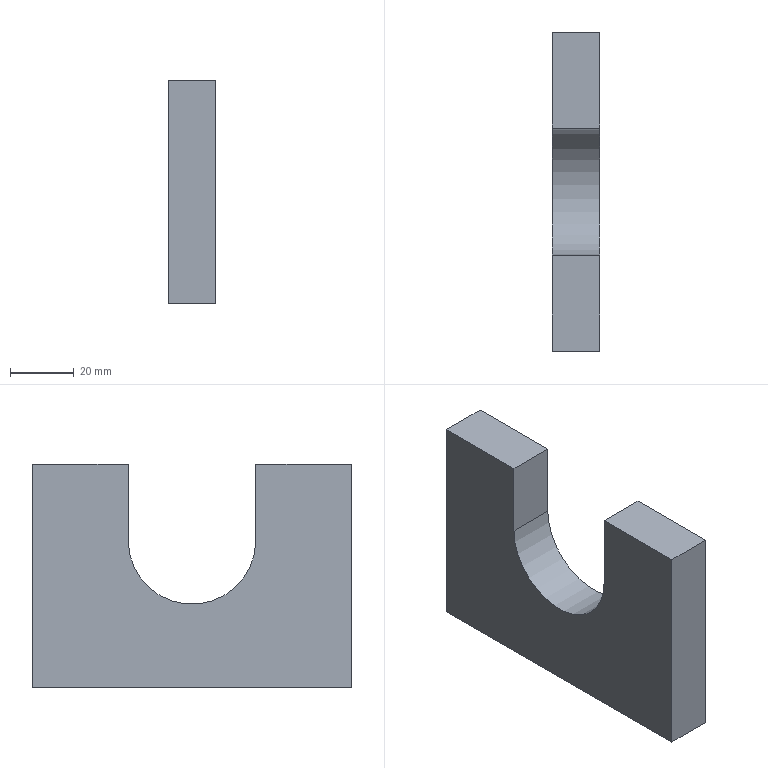Part | STEP file | Tube feed_id678_x_t | 1 solid | 10 faces | box 15 x 100 x 70 mm | volume 81265 mm3 | plane 9 | cylinder 1 | commonest cylinder face diameters 40 x1
STEP:
#1=CARTESIAN_POINT('',(0.,0.,0.));
#2=DIRECTION('',(0.,0.,1.));
#3=DIRECTION('',(1.,0.,0.));
#4=AXIS2_PLACEMENT_3D('',#1,#2,#3);
#5=CARTESIAN_POINT('',(211.,190.936,-4.));
#6=VERTEX_POINT('',#5);
#7=CARTESIAN_POINT('',(211.,190.936,19.85));
#8=VERTEX_POINT('',#7);
#9=CARTESIAN_POINT('',(211.,190.936,12.));
#10=DIRECTION('',(0.,0.,1.));
#11=VECTOR('',#10,1.);
#12=LINE('',#9,#11);
#13=CARTESIAN_POINT('',(211.,245.936,19.85));
#14=DIRECTION('',(1.,0.,0.));
#15=DIRECTION('',(0.,0.,-1.));
#16=AXIS2_PLACEMENT_3D('',#13,#14,#15);
#17=PLANE('',#16);
#18=CARTESIAN_POINT('',(7.85,-55.));
#19=DIRECTION('',(-1.,0.));
#20=VECTOR('',#19,1.);
#21=LINE('',#18,#20);
#22=(GEOMETRIC_REPRESENTATION_CONTEXT(2)PARAMETRIC_REPRESENTATION_CONTEXT()REPRESENTATION_CONTEXT('',''));
#23=DEFINITIONAL_REPRESENTATION('',(#21),#22);
#24=PCURVE('',#17,#23);
#25=CARTESIAN_POINT('',(218.5,190.936,12.));
#26=DIRECTION('',(0.,-1.,0.));
#27=DIRECTION('',(0.,0.,-1.));
#28=AXIS2_PLACEMENT_3D('',#25,#26,#27);
#29=PLANE('',#28);
#30=CARTESIAN_POINT('',(0.,-7.5));
#31=DIRECTION('',(-1.,0.));
#32=VECTOR('',#31,1.);
#33=LINE('',#30,#32);
#34=(GEOMETRIC_REPRESENTATION_CONTEXT(2)PARAMETRIC_REPRESENTATION_CONTEXT()REPRESENTATION_CONTEXT('',''));
#35=DEFINITIONAL_REPRESENTATION('',(#33),#34);
#36=PCURVE('',#29,#35);
#37=SURFACE_CURVE('',#12,(#24,#36),.PCURVE_S1.);
#38=EDGE_CURVE('',#6,#8,#37,.T.);
#39=ORIENTED_EDGE('',*,*,#38,.F.);
#40=CARTESIAN_POINT('',(211.,230.936,-4.));
#41=VERTEX_POINT('',#40);
#42=CARTESIAN_POINT('',(211.,210.936,-4.));
#43=DIRECTION('',(-1.,0.,0.));
#44=DIRECTION('',(0.,0.,-1.));
#45=AXIS2_PLACEMENT_3D('',#42,#43,#44);
#46=CIRCLE('',#45,20.);
#47=CARTESIAN_POINT('',(43.85,-35.));
#48=CARTESIAN_POINT('',(43.85,-69.641));
#49=CARTESIAN_POINT('',(13.85,-52.321));
#50=CARTESIAN_POINT('',(-16.15,-35.));
#51=CARTESIAN_POINT('',(13.85,-17.679));
#52=CARTESIAN_POINT('',(43.85,-0.359));
#53=CARTESIAN_POINT('',(43.85,-35.));
#54=(BOUNDED_CURVE()B_SPLINE_CURVE(2,(#47,#48,#49,#50,#51,#52,#53),.UNSPECIFIED.,.T.,.F.)B_SPLINE_CURVE_WITH_KNOTS((1,2,2,2,2,1),(-2.094,0.,2.094,4.189,6.283,8.378),.UNSPECIFIED.)CURVE()GEOMETRIC_REPRESENTATION_ITEM()RATIONAL_B_SPLINE_CURVE((1.,0.5,1.,0.5,1.,0.5,1.))REPRESENTATION_ITEM(''));
#55=(GEOMETRIC_REPRESENTATION_CONTEXT(2)PARAMETRIC_REPRESENTATION_CONTEXT()REPRESENTATION_CONTEXT('',''));
#56=DEFINITIONAL_REPRESENTATION('',(#54),#55);
#57=PCURVE('',#17,#56);
#58=CARTESIAN_POINT('',(211.,210.936,-4.));
#59=DIRECTION('',(1.,0.,0.));
#60=DIRECTION('',(0.,0.,-1.));
#61=AXIS2_PLACEMENT_3D('',#58,#59,#60);
#62=CYLINDRICAL_SURFACE('',#61,20.);
#63=CARTESIAN_POINT('',(12.566,0.));
#64=DIRECTION('',(-1.,0.));
#65=VECTOR('',#64,1.);
#66=LINE('',#63,#65);
#67=(GEOMETRIC_REPRESENTATION_CONTEXT(2)PARAMETRIC_REPRESENTATION_CONTEXT()REPRESENTATION_CONTEXT('',''));
#68=DEFINITIONAL_REPRESENTATION('',(#66),#67);
#69=PCURVE('',#62,#68);
#70=SURFACE_CURVE('',#46,(#57,#69),.PCURVE_S1.);
#71=EDGE_CURVE('',#41,#6,#70,.T.);
#72=ORIENTED_EDGE('',*,*,#71,.F.);
#73=CARTESIAN_POINT('',(211.,230.936,19.85));
#74=VERTEX_POINT('',#73);
#75=CARTESIAN_POINT('',(211.,230.936,19.85));
#76=DIRECTION('',(0.,0.,1.));
#77=VECTOR('',#76,1.);
#78=LINE('',#75,#77);
#79=CARTESIAN_POINT('',(0.,-15.));
#80=DIRECTION('',(-1.,0.));
#81=VECTOR('',#80,1.);
#82=LINE('',#79,#81);
#83=(GEOMETRIC_REPRESENTATION_CONTEXT(2)PARAMETRIC_REPRESENTATION_CONTEXT()REPRESENTATION_CONTEXT('',''));
#84=DEFINITIONAL_REPRESENTATION('',(#82),#83);
#85=PCURVE('',#17,#84);
#86=CARTESIAN_POINT('',(218.5,230.936,12.));
#87=DIRECTION('',(0.,1.,0.));
#88=DIRECTION('',(0.,0.,1.));
#89=AXIS2_PLACEMENT_3D('',#86,#87,#88);
#90=PLANE('',#89);
#91=CARTESIAN_POINT('',(7.85,-7.5));
#92=DIRECTION('',(1.,0.));
#93=VECTOR('',#92,1.);
#94=LINE('',#91,#93);
#95=(GEOMETRIC_REPRESENTATION_CONTEXT(2)PARAMETRIC_REPRESENTATION_CONTEXT()REPRESENTATION_CONTEXT('',''));
#96=DEFINITIONAL_REPRESENTATION('',(#94),#95);
#97=PCURVE('',#90,#96);
#98=SURFACE_CURVE('',#78,(#85,#97),.PCURVE_S1.);
#99=EDGE_CURVE('',#41,#74,#98,.T.);
#100=ORIENTED_EDGE('',*,*,#99,.T.);
#101=CARTESIAN_POINT('',(211.,260.936,19.85));
#102=VERTEX_POINT('',#101);
#103=CARTESIAN_POINT('',(211.,175.936,19.85));
#104=DIRECTION('',(0.,-1.,0.));
#105=VECTOR('',#104,1.);
#106=LINE('',#103,#105);
#107=CARTESIAN_POINT('',(0.,-70.));
#108=DIRECTION('',(0.,-1.));
#109=VECTOR('',#108,1.);
#110=LINE('',#107,#109);
#111=(GEOMETRIC_REPRESENTATION_CONTEXT(2)PARAMETRIC_REPRESENTATION_CONTEXT()REPRESENTATION_CONTEXT('',''));
#112=DEFINITIONAL_REPRESENTATION('',(#110),#111);
#113=PCURVE('',#17,#112);
#114=CARTESIAN_POINT('',(0.,0.,19.85));
#115=DIRECTION('',(0.,0.,1.));
#116=DIRECTION('',(1.,0.,0.));
#117=AXIS2_PLACEMENT_3D('',#114,#115,#116);
#118=PLANE('',#117);
#119=CARTESIAN_POINT('',(211.,175.936));
#120=DIRECTION('',(0.,-1.));
#121=VECTOR('',#120,1.);
#122=LINE('',#119,#121);
#123=(GEOMETRIC_REPRESENTATION_CONTEXT(2)PARAMETRIC_REPRESENTATION_CONTEXT()REPRESENTATION_CONTEXT('',''));
#124=DEFINITIONAL_REPRESENTATION('',(#122),#123);
#125=PCURVE('',#118,#124);
#126=SURFACE_CURVE('',#106,(#113,#125),.PCURVE_S1.);
#127=EDGE_CURVE('',#102,#74,#126,.T.);
#128=ORIENTED_EDGE('',*,*,#127,.F.);
#129=CARTESIAN_POINT('',(211.,260.936,-50.15));
#130=VERTEX_POINT('',#129);
#131=CARTESIAN_POINT('',(211.,260.936,19.85));
#132=DIRECTION('',(0.,0.,-1.));
#133=VECTOR('',#132,1.);
#134=LINE('',#131,#133);
#135=CARTESIAN_POINT('',(0.,15.));
#136=DIRECTION('',(1.,0.));
#137=VECTOR('',#136,1.);
#138=LINE('',#135,#137);
#139=(GEOMETRIC_REPRESENTATION_CONTEXT(2)PARAMETRIC_REPRESENTATION_CONTEXT()REPRESENTATION_CONTEXT('',''));
#140=DEFINITIONAL_REPRESENTATION('',(#138),#139);
#141=PCURVE('',#17,#140);
#142=CARTESIAN_POINT('',(226.,260.936,19.85));
#143=DIRECTION('',(0.,-1.,0.));
#144=DIRECTION('',(0.,0.,-1.));
#145=AXIS2_PLACEMENT_3D('',#142,#143,#144);
#146=PLANE('',#145);
#147=CARTESIAN_POINT('',(0.,-15.));
#148=DIRECTION('',(1.,0.));
#149=VECTOR('',#148,1.);
#150=LINE('',#147,#149);
#151=(GEOMETRIC_REPRESENTATION_CONTEXT(2)PARAMETRIC_REPRESENTATION_CONTEXT()REPRESENTATION_CONTEXT('',''));
#152=DEFINITIONAL_REPRESENTATION('',(#150),#151);
#153=PCURVE('',#146,#152);
#154=SURFACE_CURVE('',#134,(#141,#153),.PCURVE_S1.);
#155=EDGE_CURVE('',#102,#130,#154,.T.);
#156=ORIENTED_EDGE('',*,*,#155,.T.);
#157=CARTESIAN_POINT('',(211.,160.936,-50.15));
#158=VERTEX_POINT('',#157);
#159=CARTESIAN_POINT('',(211.,245.936,-50.15));
#160=DIRECTION('',(0.,-1.,0.));
#161=VECTOR('',#160,1.);
#162=LINE('',#159,#161);
#163=CARTESIAN_POINT('',(70.,0.));
#164=DIRECTION('',(0.,-1.));
#165=VECTOR('',#164,1.);
#166=LINE('',#163,#165);
#167=(GEOMETRIC_REPRESENTATION_CONTEXT(2)PARAMETRIC_REPRESENTATION_CONTEXT()REPRESENTATION_CONTEXT('',''));
#168=DEFINITIONAL_REPRESENTATION('',(#166),#167);
#169=PCURVE('',#17,#168);
#170=CARTESIAN_POINT('',(0.,0.,-50.15));
#171=DIRECTION('',(0.,0.,1.));
#172=DIRECTION('',(1.,0.,0.));
#173=AXIS2_PLACEMENT_3D('',#170,#171,#172);
#174=PLANE('',#173);
#175=CARTESIAN_POINT('',(211.,245.936));
#176=DIRECTION('',(0.,-1.));
#177=VECTOR('',#176,1.);
#178=LINE('',#175,#177);
#179=(GEOMETRIC_REPRESENTATION_CONTEXT(2)PARAMETRIC_REPRESENTATION_CONTEXT()REPRESENTATION_CONTEXT('',''));
#180=DEFINITIONAL_REPRESENTATION('',(#178),#179);
#181=PCURVE('',#174,#180);
#182=SURFACE_CURVE('',#162,(#169,#181),.PCURVE_S1.);
#183=EDGE_CURVE('',#130,#158,#182,.T.);
#184=ORIENTED_EDGE('',*,*,#183,.T.);
#185=CARTESIAN_POINT('',(211.,160.936,19.85));
#186=VERTEX_POINT('',#185);
#187=CARTESIAN_POINT('',(211.,160.936,19.85));
#188=DIRECTION('',(0.,0.,-1.));
#189=VECTOR('',#188,1.);
#190=LINE('',#187,#189);
#191=CARTESIAN_POINT('',(0.,-85.));
#192=DIRECTION('',(1.,0.));
#193=VECTOR('',#192,1.);
#194=LINE('',#191,#193);
#195=(GEOMETRIC_REPRESENTATION_CONTEXT(2)PARAMETRIC_REPRESENTATION_CONTEXT()REPRESENTATION_CONTEXT('',''));
#196=DEFINITIONAL_REPRESENTATION('',(#194),#195);
#197=PCURVE('',#17,#196);
#198=CARTESIAN_POINT('',(211.,160.936,19.85));
#199=DIRECTION('',(0.,1.,0.));
#200=DIRECTION('',(0.,0.,1.));
#201=AXIS2_PLACEMENT_3D('',#198,#199,#200);
#202=PLANE('',#201);
#203=CARTESIAN_POINT('',(0.,0.));
#204=DIRECTION('',(-1.,0.));
#205=VECTOR('',#204,1.);
#206=LINE('',#203,#205);
#207=(GEOMETRIC_REPRESENTATION_CONTEXT(2)PARAMETRIC_REPRESENTATION_CONTEXT()REPRESENTATION_CONTEXT('',''));
#208=DEFINITIONAL_REPRESENTATION('',(#206),#207);
#209=PCURVE('',#202,#208);
#210=SURFACE_CURVE('',#190,(#197,#209),.PCURVE_S1.);
#211=EDGE_CURVE('',#186,#158,#210,.T.);
#212=ORIENTED_EDGE('',*,*,#211,.F.);
#213=CARTESIAN_POINT('',(211.,175.936,19.85));
#214=DIRECTION('',(0.,-1.,0.));
#215=VECTOR('',#214,1.);
#216=LINE('',#213,#215);
#217=CARTESIAN_POINT('',(0.,-70.));
#218=DIRECTION('',(0.,-1.));
#219=VECTOR('',#218,1.);
#220=LINE('',#217,#219);
#221=(GEOMETRIC_REPRESENTATION_CONTEXT(2)PARAMETRIC_REPRESENTATION_CONTEXT()REPRESENTATION_CONTEXT('',''));
#222=DEFINITIONAL_REPRESENTATION('',(#220),#221);
#223=PCURVE('',#17,#222);
#224=CARTESIAN_POINT('',(0.,0.,19.85));
#225=DIRECTION('',(0.,0.,1.));
#226=DIRECTION('',(1.,0.,0.));
#227=AXIS2_PLACEMENT_3D('',#224,#225,#226);
#228=PLANE('',#227);
#229=CARTESIAN_POINT('',(211.,175.936));
#230=DIRECTION('',(0.,-1.));
#231=VECTOR('',#230,1.);
#232=LINE('',#229,#231);
#233=(GEOMETRIC_REPRESENTATION_CONTEXT(2)PARAMETRIC_REPRESENTATION_CONTEXT()REPRESENTATION_CONTEXT('',''));
#234=DEFINITIONAL_REPRESENTATION('',(#232),#233);
#235=PCURVE('',#228,#234);
#236=SURFACE_CURVE('',#216,(#223,#235),.PCURVE_S1.);
#237=EDGE_CURVE('',#8,#186,#236,.T.);
#238=ORIENTED_EDGE('',*,*,#237,.F.);
#239=EDGE_LOOP('',(#39,#72,#100,#128,#156,#184,#212,#238));
#240=FACE_BOUND('',#239,.T.);
#241=ADVANCED_FACE('',(#240),#17,.F.);
#242=CARTESIAN_POINT('',(226.,230.936,-4.));
#243=VERTEX_POINT('',#242);
#244=CARTESIAN_POINT('',(226.,230.936,19.85));
#245=VERTEX_POINT('',#244);
#246=CARTESIAN_POINT('',(226.,230.936,12.));
#247=DIRECTION('',(0.,0.,1.));
#248=VECTOR('',#247,1.);
#249=LINE('',#246,#248);
#250=CARTESIAN_POINT('',(226.,160.936,19.85));
#251=DIRECTION('',(-1.,0.,0.));
#252=DIRECTION('',(0.,0.,1.));
#253=AXIS2_PLACEMENT_3D('',#250,#251,#252);
#254=PLANE('',#253);
#255=CARTESIAN_POINT('',(-7.85,70.));
#256=DIRECTION('',(1.,0.));
#257=VECTOR('',#256,1.);
#258=LINE('',#255,#257);
#259=(GEOMETRIC_REPRESENTATION_CONTEXT(2)PARAMETRIC_REPRESENTATION_CONTEXT()REPRESENTATION_CONTEXT('',''));
#260=DEFINITIONAL_REPRESENTATION('',(#258),#259);
#261=PCURVE('',#254,#260);
#262=CARTESIAN_POINT('',(0.,7.5));
#263=DIRECTION('',(1.,0.));
#264=VECTOR('',#263,1.);
#265=LINE('',#262,#264);
#266=(GEOMETRIC_REPRESENTATION_CONTEXT(2)PARAMETRIC_REPRESENTATION_CONTEXT()REPRESENTATION_CONTEXT('',''));
#267=DEFINITIONAL_REPRESENTATION('',(#265),#266);
#268=PCURVE('',#90,#267);
#269=SURFACE_CURVE('',#249,(#261,#268),.PCURVE_S1.);
#270=EDGE_CURVE('',#243,#245,#269,.T.);
#271=ORIENTED_EDGE('',*,*,#270,.F.);
#272=CARTESIAN_POINT('',(226.,190.936,-4.));
#273=VERTEX_POINT('',#272);
#274=CARTESIAN_POINT('',(226.,210.936,-4.));
#275=DIRECTION('',(-1.,0.,0.));
#276=DIRECTION('',(0.,0.,1.));
#277=AXIS2_PLACEMENT_3D('',#274,#275,#276);
#278=CIRCLE('',#277,20.);
#279=CARTESIAN_POINT('',(-23.85,50.));
#280=DIRECTION('',(1.,0.));
#281=AXIS2_PLACEMENT_2D('',#279,#280);
#282=CIRCLE('',#281,20.);
#283=(GEOMETRIC_REPRESENTATION_CONTEXT(2)PARAMETRIC_REPRESENTATION_CONTEXT()REPRESENTATION_CONTEXT('',''));
#284=DEFINITIONAL_REPRESENTATION('',(#282),#283);
#285=PCURVE('',#254,#284);
#286=CARTESIAN_POINT('',(9.425,15.));
#287=DIRECTION('',(-1.,0.));
#288=VECTOR('',#287,1.);
#289=LINE('',#286,#288);
#290=(GEOMETRIC_REPRESENTATION_CONTEXT(2)PARAMETRIC_REPRESENTATION_CONTEXT()REPRESENTATION_CONTEXT('',''));
#291=DEFINITIONAL_REPRESENTATION('',(#289),#290);
#292=PCURVE('',#62,#291);
#293=SURFACE_CURVE('',#278,(#285,#292),.PCURVE_S1.);
#294=EDGE_CURVE('',#243,#273,#293,.T.);
#295=ORIENTED_EDGE('',*,*,#294,.T.);
#296=CARTESIAN_POINT('',(226.,190.936,19.85));
#297=VERTEX_POINT('',#296);
#298=CARTESIAN_POINT('',(226.,190.936,19.85));
#299=DIRECTION('',(0.,0.,1.));
#300=VECTOR('',#299,1.);
#301=LINE('',#298,#300);
#302=CARTESIAN_POINT('',(0.,30.));
#303=DIRECTION('',(1.,0.));
#304=VECTOR('',#303,1.);
#305=LINE('',#302,#304);
#306=(GEOMETRIC_REPRESENTATION_CONTEXT(2)PARAMETRIC_REPRESENTATION_CONTEXT()REPRESENTATION_CONTEXT('',''));
#307=DEFINITIONAL_REPRESENTATION('',(#305),#306);
#308=PCURVE('',#254,#307);
#309=CARTESIAN_POINT('',(-7.85,7.5));
#310=DIRECTION('',(-1.,0.));
#311=VECTOR('',#310,1.);
#312=LINE('',#309,#311);
#313=(GEOMETRIC_REPRESENTATION_CONTEXT(2)PARAMETRIC_REPRESENTATION_CONTEXT()REPRESENTATION_CONTEXT('',''));
#314=DEFINITIONAL_REPRESENTATION('',(#312),#313);
#315=PCURVE('',#29,#314);
#316=SURFACE_CURVE('',#301,(#308,#315),.PCURVE_S1.);
#317=EDGE_CURVE('',#273,#297,#316,.T.);
#318=ORIENTED_EDGE('',*,*,#317,.T.);
#319=CARTESIAN_POINT('',(226.,160.936,19.85));
#320=VERTEX_POINT('',#319);
#321=CARTESIAN_POINT('',(226.,160.936,19.85));
#322=DIRECTION('',(0.,1.,0.));
#323=VECTOR('',#322,1.);
#324=LINE('',#321,#323);
#325=CARTESIAN_POINT('',(0.,0.));
#326=DIRECTION('',(0.,1.));
#327=VECTOR('',#326,1.);
#328=LINE('',#325,#327);
#329=(GEOMETRIC_REPRESENTATION_CONTEXT(2)PARAMETRIC_REPRESENTATION_CONTEXT()REPRESENTATION_CONTEXT('',''));
#330=DEFINITIONAL_REPRESENTATION('',(#328),#329);
#331=PCURVE('',#254,#330);
#332=CARTESIAN_POINT('',(226.,160.936));
#333=DIRECTION('',(0.,1.));
#334=VECTOR('',#333,1.);
#335=LINE('',#332,#334);
#336=(GEOMETRIC_REPRESENTATION_CONTEXT(2)PARAMETRIC_REPRESENTATION_CONTEXT()REPRESENTATION_CONTEXT('',''));
#337=DEFINITIONAL_REPRESENTATION('',(#335),#336);
#338=PCURVE('',#228,#337);
#339=SURFACE_CURVE('',#324,(#331,#338),.PCURVE_S1.);
#340=EDGE_CURVE('',#320,#297,#339,.T.);
#341=ORIENTED_EDGE('',*,*,#340,.F.);
#342=CARTESIAN_POINT('',(226.,160.936,-50.15));
#343=VERTEX_POINT('',#342);
#344=CARTESIAN_POINT('',(226.,160.936,19.85));
#345=DIRECTION('',(0.,0.,-1.));
#346=VECTOR('',#345,1.);
#347=LINE('',#344,#346);
#348=CARTESIAN_POINT('',(0.,0.));
#349=DIRECTION('',(-1.,0.));
#350=VECTOR('',#349,1.);
#351=LINE('',#348,#350);
#352=(GEOMETRIC_REPRESENTATION_CONTEXT(2)PARAMETRIC_REPRESENTATION_CONTEXT()REPRESENTATION_CONTEXT('',''));
#353=DEFINITIONAL_REPRESENTATION('',(#351),#352);
#354=PCURVE('',#254,#353);
#355=CARTESIAN_POINT('',(0.,15.));
#356=DIRECTION('',(-1.,0.));
#357=VECTOR('',#356,1.);
#358=LINE('',#355,#357);
#359=(GEOMETRIC_REPRESENTATION_CONTEXT(2)PARAMETRIC_REPRESENTATION_CONTEXT()REPRESENTATION_CONTEXT('',''));
#360=DEFINITIONAL_REPRESENTATION('',(#358),#359);
#361=PCURVE('',#202,#360);
#362=SURFACE_CURVE('',#347,(#354,#361),.PCURVE_S1.);
#363=EDGE_CURVE('',#320,#343,#362,.T.);
#364=ORIENTED_EDGE('',*,*,#363,.T.);
#365=CARTESIAN_POINT('',(226.,260.936,-50.15));
#366=VERTEX_POINT('',#365);
#367=CARTESIAN_POINT('',(226.,160.936,-50.15));
#368=DIRECTION('',(0.,1.,0.));
#369=VECTOR('',#368,1.);
#370=LINE('',#367,#369);
#371=CARTESIAN_POINT('',(-70.,0.));
#372=DIRECTION('',(0.,1.));
#373=VECTOR('',#372,1.);
#374=LINE('',#371,#373);
#375=(GEOMETRIC_REPRESENTATION_CONTEXT(2)PARAMETRIC_REPRESENTATION_CONTEXT()REPRESENTATION_CONTEXT('',''));
#376=DEFINITIONAL_REPRESENTATION('',(#374),#375);
#377=PCURVE('',#254,#376);
#378=CARTESIAN_POINT('',(226.,160.936));
#379=DIRECTION('',(0.,1.));
#380=VECTOR('',#379,1.);
#381=LINE('',#378,#380);
#382=(GEOMETRIC_REPRESENTATION_CONTEXT(2)PARAMETRIC_REPRESENTATION_CONTEXT()REPRESENTATION_CONTEXT('',''));
#383=DEFINITIONAL_REPRESENTATION('',(#381),#382);
#384=PCURVE('',#174,#383);
#385=SURFACE_CURVE('',#370,(#377,#384),.PCURVE_S1.);
#386=EDGE_CURVE('',#343,#366,#385,.T.);
#387=ORIENTED_EDGE('',*,*,#386,.T.);
#388=CARTESIAN_POINT('',(226.,260.936,19.85));
#389=VERTEX_POINT('',#388);
#390=CARTESIAN_POINT('',(226.,260.936,19.85));
#391=DIRECTION('',(0.,0.,-1.));
#392=VECTOR('',#391,1.);
#393=LINE('',#390,#392);
#394=CARTESIAN_POINT('',(0.,100.));
#395=DIRECTION('',(-1.,0.));
#396=VECTOR('',#395,1.);
#397=LINE('',#394,#396);
#398=(GEOMETRIC_REPRESENTATION_CONTEXT(2)PARAMETRIC_REPRESENTATION_CONTEXT()REPRESENTATION_CONTEXT('',''));
#399=DEFINITIONAL_REPRESENTATION('',(#397),#398);
#400=PCURVE('',#254,#399);
#401=CARTESIAN_POINT('',(0.,0.));
#402=DIRECTION('',(1.,0.));
#403=VECTOR('',#402,1.);
#404=LINE('',#401,#403);
#405=(GEOMETRIC_REPRESENTATION_CONTEXT(2)PARAMETRIC_REPRESENTATION_CONTEXT()REPRESENTATION_CONTEXT('',''));
#406=DEFINITIONAL_REPRESENTATION('',(#404),#405);
#407=PCURVE('',#146,#406);
#408=SURFACE_CURVE('',#393,(#400,#407),.PCURVE_S1.);
#409=EDGE_CURVE('',#389,#366,#408,.T.);
#410=ORIENTED_EDGE('',*,*,#409,.F.);
#411=CARTESIAN_POINT('',(226.,160.936,19.85));
#412=DIRECTION('',(0.,1.,0.));
#413=VECTOR('',#412,1.);
#414=LINE('',#411,#413);
#415=CARTESIAN_POINT('',(0.,0.));
#416=DIRECTION('',(0.,1.));
#417=VECTOR('',#416,1.);
#418=LINE('',#415,#417);
#419=(GEOMETRIC_REPRESENTATION_CONTEXT(2)PARAMETRIC_REPRESENTATION_CONTEXT()REPRESENTATION_CONTEXT('',''));
#420=DEFINITIONAL_REPRESENTATION('',(#418),#419);
#421=PCURVE('',#254,#420);
#422=CARTESIAN_POINT('',(226.,160.936));
#423=DIRECTION('',(0.,1.));
#424=VECTOR('',#423,1.);
#425=LINE('',#422,#424);
#426=(GEOMETRIC_REPRESENTATION_CONTEXT(2)PARAMETRIC_REPRESENTATION_CONTEXT()REPRESENTATION_CONTEXT('',''));
#427=DEFINITIONAL_REPRESENTATION('',(#425),#426);
#428=PCURVE('',#118,#427);
#429=SURFACE_CURVE('',#414,(#421,#428),.PCURVE_S1.);
#430=EDGE_CURVE('',#245,#389,#429,.T.);
#431=ORIENTED_EDGE('',*,*,#430,.F.);
#432=EDGE_LOOP('',(#271,#295,#318,#341,#364,#387,#410,#431));
#433=FACE_BOUND('',#432,.T.);
#434=ADVANCED_FACE('',(#433),#254,.F.);
#435=CARTESIAN_POINT('',(0.,190.936,19.85));
#436=DIRECTION('',(1.,0.,0.));
#437=VECTOR('',#436,1.);
#438=LINE('',#435,#437);
#439=CARTESIAN_POINT('',(0.,190.936));
#440=DIRECTION('',(1.,0.));
#441=VECTOR('',#440,1.);
#442=LINE('',#439,#441);
#443=(GEOMETRIC_REPRESENTATION_CONTEXT(2)PARAMETRIC_REPRESENTATION_CONTEXT()REPRESENTATION_CONTEXT('',''));
#444=DEFINITIONAL_REPRESENTATION('',(#442),#443);
#445=PCURVE('',#228,#444);
#446=CARTESIAN_POINT('',(-7.85,-218.5));
#447=DIRECTION('',(0.,1.));
#448=VECTOR('',#447,1.);
#449=LINE('',#446,#448);
#450=(GEOMETRIC_REPRESENTATION_CONTEXT(2)PARAMETRIC_REPRESENTATION_CONTEXT()REPRESENTATION_CONTEXT('',''));
#451=DEFINITIONAL_REPRESENTATION('',(#449),#450);
#452=PCURVE('',#29,#451);
#453=SURFACE_CURVE('',#438,(#445,#452),.PCURVE_S1.);
#454=EDGE_CURVE('',#8,#297,#453,.T.);
#455=ORIENTED_EDGE('',*,*,#454,.F.);
#456=ORIENTED_EDGE('',*,*,#237,.T.);
#457=CARTESIAN_POINT('',(211.,160.936,19.85));
#458=DIRECTION('',(1.,0.,0.));
#459=VECTOR('',#458,1.);
#460=LINE('',#457,#459);
#461=CARTESIAN_POINT('',(211.,160.936));
#462=DIRECTION('',(1.,0.));
#463=VECTOR('',#462,1.);
#464=LINE('',#461,#463);
#465=(GEOMETRIC_REPRESENTATION_CONTEXT(2)PARAMETRIC_REPRESENTATION_CONTEXT()REPRESENTATION_CONTEXT('',''));
#466=DEFINITIONAL_REPRESENTATION('',(#464),#465);
#467=PCURVE('',#228,#466);
#468=CARTESIAN_POINT('',(0.,0.));
#469=DIRECTION('',(0.,1.));
#470=VECTOR('',#469,1.);
#471=LINE('',#468,#470);
#472=(GEOMETRIC_REPRESENTATION_CONTEXT(2)PARAMETRIC_REPRESENTATION_CONTEXT()REPRESENTATION_CONTEXT('',''));
#473=DEFINITIONAL_REPRESENTATION('',(#471),#472);
#474=PCURVE('',#202,#473);
#475=SURFACE_CURVE('',#460,(#467,#474),.PCURVE_S1.);
#476=EDGE_CURVE('',#186,#320,#475,.T.);
#477=ORIENTED_EDGE('',*,*,#476,.T.);
#478=ORIENTED_EDGE('',*,*,#340,.T.);
#479=EDGE_LOOP('',(#455,#456,#477,#478));
#480=FACE_BOUND('',#479,.T.);
#481=ADVANCED_FACE('',(#480),#228,.T.);
#482=CARTESIAN_POINT('',(211.,160.936,-50.15));
#483=DIRECTION('',(1.,0.,0.));
#484=VECTOR('',#483,1.);
#485=LINE('',#482,#484);
#486=CARTESIAN_POINT('',(-70.,0.));
#487=DIRECTION('',(0.,1.));
#488=VECTOR('',#487,1.);
#489=LINE('',#486,#488);
#490=(GEOMETRIC_REPRESENTATION_CONTEXT(2)PARAMETRIC_REPRESENTATION_CONTEXT()REPRESENTATION_CONTEXT('',''));
#491=DEFINITIONAL_REPRESENTATION('',(#489),#490);
#492=PCURVE('',#202,#491);
#493=CARTESIAN_POINT('',(211.,160.936));
#494=DIRECTION('',(1.,0.));
#495=VECTOR('',#494,1.);
#496=LINE('',#493,#495);
#497=(GEOMETRIC_REPRESENTATION_CONTEXT(2)PARAMETRIC_REPRESENTATION_CONTEXT()REPRESENTATION_CONTEXT('',''));
#498=DEFINITIONAL_REPRESENTATION('',(#496),#497);
#499=PCURVE('',#174,#498);
#500=SURFACE_CURVE('',#485,(#492,#499),.PCURVE_S1.);
#501=EDGE_CURVE('',#158,#343,#500,.T.);
#502=ORIENTED_EDGE('',*,*,#501,.T.);
#503=ORIENTED_EDGE('',*,*,#363,.F.);
#504=ORIENTED_EDGE('',*,*,#476,.F.);
#505=ORIENTED_EDGE('',*,*,#211,.T.);
#506=EDGE_LOOP('',(#502,#503,#504,#505));
#507=FACE_BOUND('',#506,.T.);
#508=ADVANCED_FACE('',(#507),#202,.F.);
#509=CARTESIAN_POINT('',(226.,260.936,-50.15));
#510=DIRECTION('',(-1.,0.,0.));
#511=VECTOR('',#510,1.);
#512=LINE('',#509,#511);
#513=CARTESIAN_POINT('',(70.,0.));
#514=DIRECTION('',(0.,-1.));
#515=VECTOR('',#514,1.);
#516=LINE('',#513,#515);
#517=(GEOMETRIC_REPRESENTATION_CONTEXT(2)PARAMETRIC_REPRESENTATION_CONTEXT()REPRESENTATION_CONTEXT('',''));
#518=DEFINITIONAL_REPRESENTATION('',(#516),#517);
#519=PCURVE('',#146,#518);
#520=CARTESIAN_POINT('',(226.,260.936));
#521=DIRECTION('',(-1.,0.));
#522=VECTOR('',#521,1.);
#523=LINE('',#520,#522);
#524=(GEOMETRIC_REPRESENTATION_CONTEXT(2)PARAMETRIC_REPRESENTATION_CONTEXT()REPRESENTATION_CONTEXT('',''));
#525=DEFINITIONAL_REPRESENTATION('',(#523),#524);
#526=PCURVE('',#174,#525);
#527=SURFACE_CURVE('',#512,(#519,#526),.PCURVE_S1.);
#528=EDGE_CURVE('',#366,#130,#527,.T.);
#529=ORIENTED_EDGE('',*,*,#528,.T.);
#530=ORIENTED_EDGE('',*,*,#155,.F.);
#531=CARTESIAN_POINT('',(226.,260.936,19.85));
#532=DIRECTION('',(-1.,0.,0.));
#533=VECTOR('',#532,1.);
#534=LINE('',#531,#533);
#535=CARTESIAN_POINT('',(0.,0.));
#536=DIRECTION('',(0.,-1.));
#537=VECTOR('',#536,1.);
#538=LINE('',#535,#537);
#539=(GEOMETRIC_REPRESENTATION_CONTEXT(2)PARAMETRIC_REPRESENTATION_CONTEXT()REPRESENTATION_CONTEXT('',''));
#540=DEFINITIONAL_REPRESENTATION('',(#538),#539);
#541=PCURVE('',#146,#540);
#542=CARTESIAN_POINT('',(226.,260.936));
#543=DIRECTION('',(-1.,0.));
#544=VECTOR('',#543,1.);
#545=LINE('',#542,#544);
#546=(GEOMETRIC_REPRESENTATION_CONTEXT(2)PARAMETRIC_REPRESENTATION_CONTEXT()REPRESENTATION_CONTEXT('',''));
#547=DEFINITIONAL_REPRESENTATION('',(#545),#546);
#548=PCURVE('',#118,#547);
#549=SURFACE_CURVE('',#534,(#541,#548),.PCURVE_S1.);
#550=EDGE_CURVE('',#389,#102,#549,.T.);
#551=ORIENTED_EDGE('',*,*,#550,.F.);
#552=ORIENTED_EDGE('',*,*,#409,.T.);
#553=EDGE_LOOP('',(#529,#530,#551,#552));
#554=FACE_BOUND('',#553,.T.);
#555=ADVANCED_FACE('',(#554),#146,.F.);
#556=CARTESIAN_POINT('',(0.,230.936,19.85));
#557=DIRECTION('',(-1.,0.,0.));
#558=VECTOR('',#557,1.);
#559=LINE('',#556,#558);
#560=CARTESIAN_POINT('',(0.,230.936));
#561=DIRECTION('',(-1.,0.));
#562=VECTOR('',#561,1.);
#563=LINE('',#560,#562);
#564=(GEOMETRIC_REPRESENTATION_CONTEXT(2)PARAMETRIC_REPRESENTATION_CONTEXT()REPRESENTATION_CONTEXT('',''));
#565=DEFINITIONAL_REPRESENTATION('',(#563),#564);
#566=PCURVE('',#118,#565);
#567=CARTESIAN_POINT('',(7.85,-218.5));
#568=DIRECTION('',(0.,-1.));
#569=VECTOR('',#568,1.);
#570=LINE('',#567,#569);
#571=(GEOMETRIC_REPRESENTATION_CONTEXT(2)PARAMETRIC_REPRESENTATION_CONTEXT()REPRESENTATION_CONTEXT('',''));
#572=DEFINITIONAL_REPRESENTATION('',(#570),#571);
#573=PCURVE('',#90,#572);
#574=SURFACE_CURVE('',#559,(#566,#573),.PCURVE_S1.);
#575=EDGE_CURVE('',#245,#74,#574,.T.);
#576=ORIENTED_EDGE('',*,*,#575,.F.);
#577=ORIENTED_EDGE('',*,*,#430,.T.);
#578=ORIENTED_EDGE('',*,*,#550,.T.);
#579=ORIENTED_EDGE('',*,*,#127,.T.);
#580=EDGE_LOOP('',(#576,#577,#578,#579));
#581=FACE_BOUND('',#580,.T.);
#582=ADVANCED_FACE('',(#581),#118,.T.);
#583=ORIENTED_EDGE('',*,*,#501,.F.);
#584=ORIENTED_EDGE('',*,*,#183,.F.);
#585=ORIENTED_EDGE('',*,*,#528,.F.);
#586=ORIENTED_EDGE('',*,*,#386,.F.);
#587=EDGE_LOOP('',(#583,#584,#585,#586));
#588=FACE_BOUND('',#587,.T.);
#589=ADVANCED_FACE('',(#588),#174,.F.);
#590=ORIENTED_EDGE('',*,*,#454,.T.);
#591=ORIENTED_EDGE('',*,*,#317,.F.);
#592=CARTESIAN_POINT('',(218.5,190.936,-4.));
#593=DIRECTION('',(-1.,0.,0.));
#594=VECTOR('',#593,1.);
#595=LINE('',#592,#594);
#596=CARTESIAN_POINT('',(16.,0.));
#597=DIRECTION('',(0.,-1.));
#598=VECTOR('',#597,1.);
#599=LINE('',#596,#598);
#600=(GEOMETRIC_REPRESENTATION_CONTEXT(2)PARAMETRIC_REPRESENTATION_CONTEXT()REPRESENTATION_CONTEXT('',''));
#601=DEFINITIONAL_REPRESENTATION('',(#599),#600);
#602=PCURVE('',#29,#601);
#603=CARTESIAN_POINT('',(4.712,7.5));
#604=DIRECTION('',(0.,-1.));
#605=VECTOR('',#604,1.);
#606=LINE('',#603,#605);
#607=(GEOMETRIC_REPRESENTATION_CONTEXT(2)PARAMETRIC_REPRESENTATION_CONTEXT()REPRESENTATION_CONTEXT('',''));
#608=DEFINITIONAL_REPRESENTATION('',(#606),#607);
#609=PCURVE('',#62,#608);
#610=SURFACE_CURVE('',#595,(#602,#609),.PCURVE_S1.);
#611=EDGE_CURVE('',#273,#6,#610,.T.);
#612=ORIENTED_EDGE('',*,*,#611,.T.);
#613=ORIENTED_EDGE('',*,*,#38,.T.);
#614=EDGE_LOOP('',(#590,#591,#612,#613));
#615=FACE_BOUND('',#614,.T.);
#616=ADVANCED_FACE('',(#615),#29,.F.);
#617=ORIENTED_EDGE('',*,*,#575,.T.);
#618=ORIENTED_EDGE('',*,*,#99,.F.);
#619=CARTESIAN_POINT('',(218.5,230.936,-4.));
#620=DIRECTION('',(1.,0.,0.));
#621=VECTOR('',#620,1.);
#622=LINE('',#619,#621);
#623=CARTESIAN_POINT('',(-16.,0.));
#624=DIRECTION('',(0.,1.));
#625=VECTOR('',#624,1.);
#626=LINE('',#623,#625);
#627=(GEOMETRIC_REPRESENTATION_CONTEXT(2)PARAMETRIC_REPRESENTATION_CONTEXT()REPRESENTATION_CONTEXT('',''));
#628=DEFINITIONAL_REPRESENTATION('',(#626),#627);
#629=PCURVE('',#90,#628);
#630=CARTESIAN_POINT('',(7.854,7.5));
#631=DIRECTION('',(0.,1.));
#632=VECTOR('',#631,1.);
#633=LINE('',#630,#632);
#634=(GEOMETRIC_REPRESENTATION_CONTEXT(2)PARAMETRIC_REPRESENTATION_CONTEXT()REPRESENTATION_CONTEXT('',''));
#635=DEFINITIONAL_REPRESENTATION('',(#633),#634);
#636=PCURVE('',#62,#635);
#637=SURFACE_CURVE('',#622,(#629,#636),.PCURVE_S1.);
#638=EDGE_CURVE('',#41,#243,#637,.T.);
#639=ORIENTED_EDGE('',*,*,#638,.T.);
#640=ORIENTED_EDGE('',*,*,#270,.T.);
#641=EDGE_LOOP('',(#617,#618,#639,#640));
#642=FACE_BOUND('',#641,.T.);
#643=ADVANCED_FACE('',(#642),#90,.F.);
#644=ORIENTED_EDGE('',*,*,#611,.T.);
#645=ORIENTED_EDGE('',*,*,#71,.F.);
#646=ORIENTED_EDGE('',*,*,#638,.T.);
#647=ORIENTED_EDGE('',*,*,#294,.T.);
#648=EDGE_LOOP('',(#644,#645,#646,#647));
#649=FACE_BOUND('',#648,.F.);
#650=ADVANCED_FACE('',(#649),#62,.F.);
#651=CLOSED_SHELL('',(#241,#434,#481,#508,#555,#582,#589,#616,#643,#650));
#652=MANIFOLD_SOLID_BREP('',#651);
#653=(LENGTH_UNIT()NAMED_UNIT(*)SI_UNIT(.MILLI.,.METRE.));
#654=UNCERTAINTY_MEASURE_WITH_UNIT(LENGTH_MEASURE(0.0000001),#653,'','');
#655=(NAMED_UNIT(*)PLANE_ANGLE_UNIT()SI_UNIT($,.RADIAN.));
#656=(NAMED_UNIT(*)SI_UNIT($,.STERADIAN.)SOLID_ANGLE_UNIT());
#657=(GEOMETRIC_REPRESENTATION_CONTEXT(3)GLOBAL_UNCERTAINTY_ASSIGNED_CONTEXT((#654))GLOBAL_UNIT_ASSIGNED_CONTEXT((#653,#655,#656))REPRESENTATION_CONTEXT('',''));
#658=ADVANCED_BREP_SHAPE_REPRESENTATION('',(#4,#652),#657);